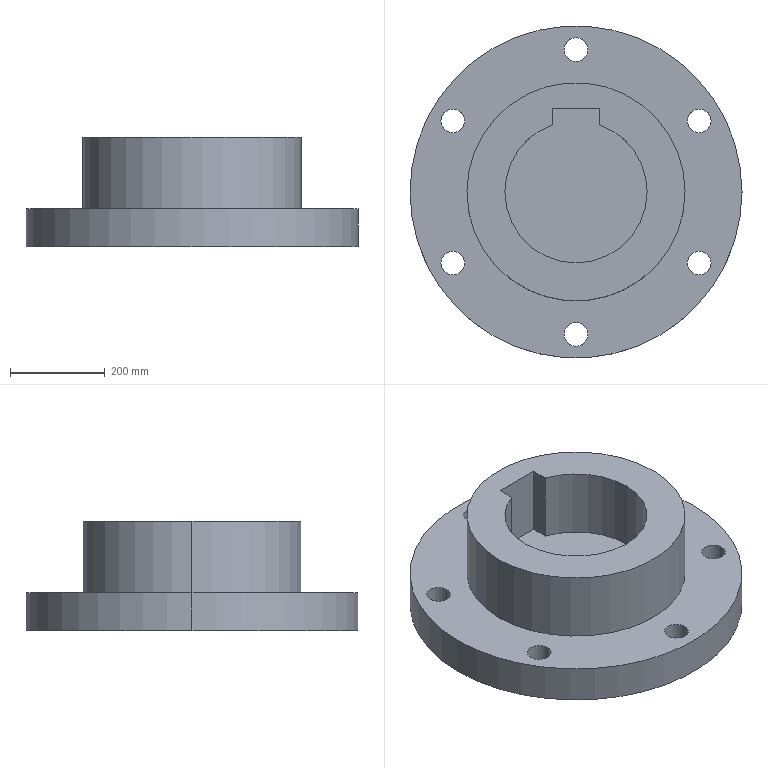Part | SolidWorks | features ICE 2, Extrusion 1 | 1 solid | 26 faces | box 700 x 700 x 230 mm | volume 43732082 mm3 | cylinder 19 | plane 7 | commonest cylinder face diameters 50 x12 300 x3 460 x2 700 x2
STEP:
#1=CARTESIAN_POINT('',(-284.808,150.,-230.));
#2=VERTEX_POINT('',#1);
#3=CARTESIAN_POINT('',(-234.808,150.,-230.));
#4=VERTEX_POINT('',#3);
#5=CARTESIAN_POINT('',(-259.808,150.,-230.));
#6=DIRECTION('',(0.,0.,1.));
#7=DIRECTION('',(-1.,0.,0.));
#8=AXIS2_PLACEMENT_3D('',#5,#6,#7);
#9=CIRCLE('',#8,25.);
#10=EDGE_CURVE('',#2,#4,#9,.T.);
#11=ORIENTED_EDGE('',*,*,#10,.F.);
#12=CARTESIAN_POINT('',(-284.808,150.,-150.));
#13=VERTEX_POINT('',#12);
#14=CARTESIAN_POINT('',(-284.808,150.,-486.));
#15=DIRECTION('',(0.,0.,1.));
#16=VECTOR('',#15,1000.);
#17=LINE('',#14,#16);
#18=EDGE_CURVE('',#2,#13,#17,.T.);
#19=ORIENTED_EDGE('',*,*,#18,.T.);
#20=CARTESIAN_POINT('',(-234.808,150.,-150.));
#21=VERTEX_POINT('',#20);
#22=CARTESIAN_POINT('',(-259.808,150.,-150.));
#23=DIRECTION('',(0.,0.,1.));
#24=DIRECTION('',(-1.,0.,0.));
#25=AXIS2_PLACEMENT_3D('',#22,#23,#24);
#26=CIRCLE('',#25,25.);
#27=EDGE_CURVE('',#13,#21,#26,.T.);
#28=ORIENTED_EDGE('',*,*,#27,.T.);
#29=CARTESIAN_POINT('',(-234.808,150.,-486.));
#30=DIRECTION('',(0.,0.,1.));
#31=VECTOR('',#30,1000.);
#32=LINE('',#29,#31);
#33=EDGE_CURVE('',#4,#21,#32,.T.);
#34=ORIENTED_EDGE('',*,*,#33,.F.);
#35=EDGE_LOOP('',(#11,#19,#28,#34));
#36=FACE_OUTER_BOUND('',#35,.T.);
#37=CARTESIAN_POINT('',(-259.808,150.,-486.));
#38=DIRECTION('',(0.,0.,1.));
#39=DIRECTION('',(1.,0.,0.));
#40=AXIS2_PLACEMENT_3D('',#37,#38,#39);
#41=CYLINDRICAL_SURFACE('',#40,25.);
#42=ADVANCED_FACE('',(#36),#41,.F.);
#43=CARTESIAN_POINT('',(-284.808,-150.,-230.));
#44=VERTEX_POINT('',#43);
#45=CARTESIAN_POINT('',(-234.808,-150.,-230.));
#46=VERTEX_POINT('',#45);
#47=CARTESIAN_POINT('',(-259.808,-150.,-230.));
#48=DIRECTION('',(0.,0.,1.));
#49=DIRECTION('',(-1.,0.,0.));
#50=AXIS2_PLACEMENT_3D('',#47,#48,#49);
#51=CIRCLE('',#50,25.);
#52=EDGE_CURVE('',#44,#46,#51,.T.);
#53=ORIENTED_EDGE('',*,*,#52,.F.);
#54=CARTESIAN_POINT('',(-284.808,-150.,-150.));
#55=VERTEX_POINT('',#54);
#56=CARTESIAN_POINT('',(-284.808,-150.,-486.));
#57=DIRECTION('',(0.,0.,1.));
#58=VECTOR('',#57,1000.);
#59=LINE('',#56,#58);
#60=EDGE_CURVE('',#44,#55,#59,.T.);
#61=ORIENTED_EDGE('',*,*,#60,.T.);
#62=CARTESIAN_POINT('',(-234.808,-150.,-150.));
#63=VERTEX_POINT('',#62);
#64=CARTESIAN_POINT('',(-259.808,-150.,-150.));
#65=DIRECTION('',(0.,0.,1.));
#66=DIRECTION('',(-1.,0.,0.));
#67=AXIS2_PLACEMENT_3D('',#64,#65,#66);
#68=CIRCLE('',#67,25.);
#69=EDGE_CURVE('',#55,#63,#68,.T.);
#70=ORIENTED_EDGE('',*,*,#69,.T.);
#71=CARTESIAN_POINT('',(-234.808,-150.,-486.));
#72=DIRECTION('',(0.,0.,1.));
#73=VECTOR('',#72,1000.);
#74=LINE('',#71,#73);
#75=EDGE_CURVE('',#46,#63,#74,.T.);
#76=ORIENTED_EDGE('',*,*,#75,.F.);
#77=EDGE_LOOP('',(#53,#61,#70,#76));
#78=FACE_OUTER_BOUND('',#77,.T.);
#79=CARTESIAN_POINT('',(-259.808,-150.,-486.));
#80=DIRECTION('',(0.,0.,1.));
#81=DIRECTION('',(1.,0.,0.));
#82=AXIS2_PLACEMENT_3D('',#79,#80,#81);
#83=CYLINDRICAL_SURFACE('',#82,25.);
#84=ADVANCED_FACE('',(#78),#83,.F.);
#85=CARTESIAN_POINT('',(-25.,-300.,-230.));
#86=VERTEX_POINT('',#85);
#87=CARTESIAN_POINT('',(25.,-300.,-230.));
#88=VERTEX_POINT('',#87);
#89=CARTESIAN_POINT('',(0.,-300.,-230.));
#90=DIRECTION('',(0.,0.,1.));
#91=DIRECTION('',(-1.,0.,0.));
#92=AXIS2_PLACEMENT_3D('',#89,#90,#91);
#93=CIRCLE('',#92,25.);
#94=EDGE_CURVE('',#86,#88,#93,.T.);
#95=ORIENTED_EDGE('',*,*,#94,.F.);
#96=CARTESIAN_POINT('',(-25.,-300.,-150.));
#97=VERTEX_POINT('',#96);
#98=CARTESIAN_POINT('',(-25.,-300.,-486.));
#99=DIRECTION('',(0.,0.,1.));
#100=VECTOR('',#99,1000.);
#101=LINE('',#98,#100);
#102=EDGE_CURVE('',#86,#97,#101,.T.);
#103=ORIENTED_EDGE('',*,*,#102,.T.);
#104=CARTESIAN_POINT('',(25.,-300.,-150.));
#105=VERTEX_POINT('',#104);
#106=CARTESIAN_POINT('',(0.,-300.,-150.));
#107=DIRECTION('',(0.,0.,1.));
#108=DIRECTION('',(-1.,0.,0.));
#109=AXIS2_PLACEMENT_3D('',#106,#107,#108);
#110=CIRCLE('',#109,25.);
#111=EDGE_CURVE('',#97,#105,#110,.T.);
#112=ORIENTED_EDGE('',*,*,#111,.T.);
#113=CARTESIAN_POINT('',(25.,-300.,-486.));
#114=DIRECTION('',(0.,0.,1.));
#115=VECTOR('',#114,1000.);
#116=LINE('',#113,#115);
#117=EDGE_CURVE('',#88,#105,#116,.T.);
#118=ORIENTED_EDGE('',*,*,#117,.F.);
#119=EDGE_LOOP('',(#95,#103,#112,#118));
#120=FACE_OUTER_BOUND('',#119,.T.);
#121=CARTESIAN_POINT('',(0.,-300.,-486.));
#122=DIRECTION('',(0.,0.,1.));
#123=DIRECTION('',(1.,0.,0.));
#124=AXIS2_PLACEMENT_3D('',#121,#122,#123);
#125=CYLINDRICAL_SURFACE('',#124,25.);
#126=ADVANCED_FACE('',(#120),#125,.F.);
#127=CARTESIAN_POINT('',(234.808,-150.,-230.));
#128=VERTEX_POINT('',#127);
#129=CARTESIAN_POINT('',(284.808,-150.,-230.));
#130=VERTEX_POINT('',#129);
#131=CARTESIAN_POINT('',(259.808,-150.,-230.));
#132=DIRECTION('',(0.,0.,1.));
#133=DIRECTION('',(-1.,0.,0.));
#134=AXIS2_PLACEMENT_3D('',#131,#132,#133);
#135=CIRCLE('',#134,25.);
#136=EDGE_CURVE('',#128,#130,#135,.T.);
#137=ORIENTED_EDGE('',*,*,#136,.F.);
#138=CARTESIAN_POINT('',(234.808,-150.,-150.));
#139=VERTEX_POINT('',#138);
#140=CARTESIAN_POINT('',(234.808,-150.,-486.));
#141=DIRECTION('',(0.,0.,1.));
#142=VECTOR('',#141,1000.);
#143=LINE('',#140,#142);
#144=EDGE_CURVE('',#128,#139,#143,.T.);
#145=ORIENTED_EDGE('',*,*,#144,.T.);
#146=CARTESIAN_POINT('',(284.808,-150.,-150.));
#147=VERTEX_POINT('',#146);
#148=CARTESIAN_POINT('',(259.808,-150.,-150.));
#149=DIRECTION('',(0.,0.,1.));
#150=DIRECTION('',(-1.,0.,0.));
#151=AXIS2_PLACEMENT_3D('',#148,#149,#150);
#152=CIRCLE('',#151,25.);
#153=EDGE_CURVE('',#139,#147,#152,.T.);
#154=ORIENTED_EDGE('',*,*,#153,.T.);
#155=CARTESIAN_POINT('',(284.808,-150.,-486.));
#156=DIRECTION('',(0.,0.,1.));
#157=VECTOR('',#156,1000.);
#158=LINE('',#155,#157);
#159=EDGE_CURVE('',#130,#147,#158,.T.);
#160=ORIENTED_EDGE('',*,*,#159,.F.);
#161=EDGE_LOOP('',(#137,#145,#154,#160));
#162=FACE_OUTER_BOUND('',#161,.T.);
#163=CARTESIAN_POINT('',(259.808,-150.,-486.));
#164=DIRECTION('',(0.,0.,1.));
#165=DIRECTION('',(1.,0.,0.));
#166=AXIS2_PLACEMENT_3D('',#163,#164,#165);
#167=CYLINDRICAL_SURFACE('',#166,25.);
#168=ADVANCED_FACE('',(#162),#167,.F.);
#169=CARTESIAN_POINT('',(234.808,150.,-230.));
#170=VERTEX_POINT('',#169);
#171=CARTESIAN_POINT('',(284.808,150.,-230.));
#172=VERTEX_POINT('',#171);
#173=CARTESIAN_POINT('',(259.808,150.,-230.));
#174=DIRECTION('',(0.,0.,1.));
#175=DIRECTION('',(-1.,0.,0.));
#176=AXIS2_PLACEMENT_3D('',#173,#174,#175);
#177=CIRCLE('',#176,25.);
#178=EDGE_CURVE('',#170,#172,#177,.T.);
#179=ORIENTED_EDGE('',*,*,#178,.F.);
#180=CARTESIAN_POINT('',(234.808,150.,-150.));
#181=VERTEX_POINT('',#180);
#182=CARTESIAN_POINT('',(234.808,150.,-486.));
#183=DIRECTION('',(0.,0.,1.));
#184=VECTOR('',#183,1000.);
#185=LINE('',#182,#184);
#186=EDGE_CURVE('',#170,#181,#185,.T.);
#187=ORIENTED_EDGE('',*,*,#186,.T.);
#188=CARTESIAN_POINT('',(284.808,150.,-150.));
#189=VERTEX_POINT('',#188);
#190=CARTESIAN_POINT('',(259.808,150.,-150.));
#191=DIRECTION('',(0.,0.,1.));
#192=DIRECTION('',(-1.,0.,0.));
#193=AXIS2_PLACEMENT_3D('',#190,#191,#192);
#194=CIRCLE('',#193,25.);
#195=EDGE_CURVE('',#181,#189,#194,.T.);
#196=ORIENTED_EDGE('',*,*,#195,.T.);
#197=CARTESIAN_POINT('',(284.808,150.,-486.));
#198=DIRECTION('',(0.,0.,1.));
#199=VECTOR('',#198,1000.);
#200=LINE('',#197,#199);
#201=EDGE_CURVE('',#172,#189,#200,.T.);
#202=ORIENTED_EDGE('',*,*,#201,.F.);
#203=EDGE_LOOP('',(#179,#187,#196,#202));
#204=FACE_OUTER_BOUND('',#203,.T.);
#205=CARTESIAN_POINT('',(259.808,150.,-486.));
#206=DIRECTION('',(0.,0.,1.));
#207=DIRECTION('',(1.,0.,0.));
#208=AXIS2_PLACEMENT_3D('',#205,#206,#207);
#209=CYLINDRICAL_SURFACE('',#208,25.);
#210=ADVANCED_FACE('',(#204),#209,.F.);
#211=CARTESIAN_POINT('',(-25.,300.,-230.));
#212=VERTEX_POINT('',#211);
#213=CARTESIAN_POINT('',(25.,300.,-230.));
#214=VERTEX_POINT('',#213);
#215=CARTESIAN_POINT('',(0.,300.,-230.));
#216=DIRECTION('',(0.,0.,1.));
#217=DIRECTION('',(-1.,0.,0.));
#218=AXIS2_PLACEMENT_3D('',#215,#216,#217);
#219=CIRCLE('',#218,25.);
#220=EDGE_CURVE('',#212,#214,#219,.T.);
#221=ORIENTED_EDGE('',*,*,#220,.F.);
#222=CARTESIAN_POINT('',(-25.,300.,-150.));
#223=VERTEX_POINT('',#222);
#224=CARTESIAN_POINT('',(-25.,300.,-486.));
#225=DIRECTION('',(0.,0.,1.));
#226=VECTOR('',#225,1000.);
#227=LINE('',#224,#226);
#228=EDGE_CURVE('',#212,#223,#227,.T.);
#229=ORIENTED_EDGE('',*,*,#228,.T.);
#230=CARTESIAN_POINT('',(25.,300.,-150.));
#231=VERTEX_POINT('',#230);
#232=CARTESIAN_POINT('',(0.,300.,-150.));
#233=DIRECTION('',(0.,0.,1.));
#234=DIRECTION('',(-1.,0.,0.));
#235=AXIS2_PLACEMENT_3D('',#232,#233,#234);
#236=CIRCLE('',#235,25.);
#237=EDGE_CURVE('',#223,#231,#236,.T.);
#238=ORIENTED_EDGE('',*,*,#237,.T.);
#239=CARTESIAN_POINT('',(25.,300.,-486.));
#240=DIRECTION('',(0.,0.,1.));
#241=VECTOR('',#240,1000.);
#242=LINE('',#239,#241);
#243=EDGE_CURVE('',#214,#231,#242,.T.);
#244=ORIENTED_EDGE('',*,*,#243,.F.);
#245=EDGE_LOOP('',(#221,#229,#238,#244));
#246=FACE_OUTER_BOUND('',#245,.T.);
#247=CARTESIAN_POINT('',(0.,300.,-486.));
#248=DIRECTION('',(0.,0.,1.));
#249=DIRECTION('',(1.,0.,0.));
#250=AXIS2_PLACEMENT_3D('',#247,#248,#249);
#251=CYLINDRICAL_SURFACE('',#250,25.);
#252=ADVANCED_FACE('',(#246),#251,.F.);
#253=CARTESIAN_POINT('',(-350.,0.,-230.));
#254=VERTEX_POINT('',#253);
#255=CARTESIAN_POINT('',(350.,0.,-230.));
#256=VERTEX_POINT('',#255);
#257=CARTESIAN_POINT('',(0.,0.,-230.));
#258=DIRECTION('',(0.,0.,-1.));
#259=DIRECTION('',(-1.,0.,0.));
#260=AXIS2_PLACEMENT_3D('',#257,#258,#259);
#261=CIRCLE('',#260,350.);
#262=EDGE_CURVE('',#254,#256,#261,.T.);
#263=ORIENTED_EDGE('',*,*,#262,.F.);
#264=CARTESIAN_POINT('',(-350.,0.,-150.));
#265=VERTEX_POINT('',#264);
#266=CARTESIAN_POINT('',(-350.,0.,-230.));
#267=DIRECTION('',(0.,0.,1.));
#268=VECTOR('',#267,1000.);
#269=LINE('',#266,#268);
#270=EDGE_CURVE('',#254,#265,#269,.T.);
#271=ORIENTED_EDGE('',*,*,#270,.T.);
#272=CARTESIAN_POINT('',(350.,0.,-150.));
#273=VERTEX_POINT('',#272);
#274=CARTESIAN_POINT('',(0.,0.,-150.));
#275=DIRECTION('',(0.,0.,-1.));
#276=DIRECTION('',(-1.,0.,0.));
#277=AXIS2_PLACEMENT_3D('',#274,#275,#276);
#278=CIRCLE('',#277,350.);
#279=EDGE_CURVE('',#265,#273,#278,.T.);
#280=ORIENTED_EDGE('',*,*,#279,.T.);
#281=CARTESIAN_POINT('',(350.,0.,-230.));
#282=DIRECTION('',(0.,0.,1.));
#283=VECTOR('',#282,1000.);
#284=LINE('',#281,#283);
#285=EDGE_CURVE('',#256,#273,#284,.T.);
#286=ORIENTED_EDGE('',*,*,#285,.F.);
#287=EDGE_LOOP('',(#263,#271,#280,#286));
#288=FACE_OUTER_BOUND('',#287,.T.);
#289=CARTESIAN_POINT('',(0.,0.,-230.));
#290=DIRECTION('',(0.,0.,1.));
#291=DIRECTION('',(1.,0.,0.));
#292=AXIS2_PLACEMENT_3D('',#289,#290,#291);
#293=CYLINDRICAL_SURFACE('',#292,350.);
#294=ADVANCED_FACE('',(#288),#293,.T.);
#295=CARTESIAN_POINT('',(-150.,0.,-150.));
#296=VERTEX_POINT('',#295);
#297=CARTESIAN_POINT('',(150.,0.,-150.));
#298=VERTEX_POINT('',#297);
#299=CARTESIAN_POINT('',(0.,0.,-150.));
#300=DIRECTION('',(0.,0.,1.));
#301=DIRECTION('',(1.,0.,0.));
#302=AXIS2_PLACEMENT_3D('',#299,#300,#301);
#303=CIRCLE('',#302,150.);
#304=EDGE_CURVE('',#296,#298,#303,.T.);
#305=ORIENTED_EDGE('',*,*,#304,.F.);
#306=CARTESIAN_POINT('',(-150.,0.,0.));
#307=VERTEX_POINT('',#306);
#308=CARTESIAN_POINT('',(-150.,0.,-150.));
#309=DIRECTION('',(0.,0.,1.));
#310=VECTOR('',#309,1000.);
#311=LINE('',#308,#310);
#312=EDGE_CURVE('',#296,#307,#311,.T.);
#313=ORIENTED_EDGE('',*,*,#312,.T.);
#314=CARTESIAN_POINT('',(150.,0.,0.));
#315=VERTEX_POINT('',#314);
#316=CARTESIAN_POINT('',(0.,0.,0.));
#317=DIRECTION('',(0.,0.,1.));
#318=DIRECTION('',(1.,0.,0.));
#319=AXIS2_PLACEMENT_3D('',#316,#317,#318);
#320=CIRCLE('',#319,150.);
#321=EDGE_CURVE('',#307,#315,#320,.T.);
#322=ORIENTED_EDGE('',*,*,#321,.T.);
#323=CARTESIAN_POINT('',(150.,0.,-150.));
#324=DIRECTION('',(0.,0.,1.));
#325=VECTOR('',#324,1000.);
#326=LINE('',#323,#325);
#327=EDGE_CURVE('',#298,#315,#326,.T.);
#328=ORIENTED_EDGE('',*,*,#327,.F.);
#329=EDGE_LOOP('',(#305,#313,#322,#328));
#330=FACE_OUTER_BOUND('',#329,.T.);
#331=CARTESIAN_POINT('',(0.,0.,-150.));
#332=DIRECTION('',(0.,0.,1.));
#333=DIRECTION('',(1.,0.,0.));
#334=AXIS2_PLACEMENT_3D('',#331,#332,#333);
#335=CYLINDRICAL_SURFACE('',#334,150.);
#336=ADVANCED_FACE('',(#330),#335,.F.);
#337=CARTESIAN_POINT('',(50.,141.421,-150.));
#338=VERTEX_POINT('',#337);
#339=CARTESIAN_POINT('',(0.,0.,-150.));
#340=DIRECTION('',(0.,0.,1.));
#341=DIRECTION('',(1.,0.,0.));
#342=AXIS2_PLACEMENT_3D('',#339,#340,#341);
#343=CIRCLE('',#342,150.);
#344=EDGE_CURVE('',#298,#338,#343,.T.);
#345=ORIENTED_EDGE('',*,*,#344,.F.);
#346=ORIENTED_EDGE('',*,*,#327,.T.);
#347=CARTESIAN_POINT('',(50.,141.421,0.));
#348=VERTEX_POINT('',#347);
#349=CARTESIAN_POINT('',(0.,0.,0.));
#350=DIRECTION('',(0.,0.,1.));
#351=DIRECTION('',(1.,0.,0.));
#352=AXIS2_PLACEMENT_3D('',#349,#350,#351);
#353=CIRCLE('',#352,150.);
#354=EDGE_CURVE('',#315,#348,#353,.T.);
#355=ORIENTED_EDGE('',*,*,#354,.T.);
#356=CARTESIAN_POINT('',(50.,141.421,-150.));
#357=DIRECTION('',(0.,0.,1.));
#358=VECTOR('',#357,1000.);
#359=LINE('',#356,#358);
#360=EDGE_CURVE('',#338,#348,#359,.T.);
#361=ORIENTED_EDGE('',*,*,#360,.F.);
#362=EDGE_LOOP('',(#345,#346,#355,#361));
#363=FACE_OUTER_BOUND('',#362,.T.);
#364=CARTESIAN_POINT('',(0.,0.,-150.));
#365=DIRECTION('',(0.,0.,1.));
#366=DIRECTION('',(1.,0.,0.));
#367=AXIS2_PLACEMENT_3D('',#364,#365,#366);
#368=CYLINDRICAL_SURFACE('',#367,150.);
#369=ADVANCED_FACE('',(#363),#368,.F.);
#370=CARTESIAN_POINT('',(230.,0.,-150.));
#371=VERTEX_POINT('',#370);
#372=CARTESIAN_POINT('',(-230.,0.,-150.));
#373=VERTEX_POINT('',#372);
#374=CARTESIAN_POINT('',(0.,0.,-150.));
#375=DIRECTION('',(0.,0.,1.));
#376=DIRECTION('',(-1.,0.,0.));
#377=AXIS2_PLACEMENT_3D('',#374,#375,#376);
#378=CIRCLE('',#377,230.);
#379=EDGE_CURVE('',#371,#373,#378,.T.);
#380=ORIENTED_EDGE('',*,*,#379,.T.);
#381=CARTESIAN_POINT('',(-230.,0.,0.));
#382=VERTEX_POINT('',#381);
#383=CARTESIAN_POINT('',(-230.,0.,-150.));
#384=DIRECTION('',(0.,0.,1.));
#385=VECTOR('',#384,1000.);
#386=LINE('',#383,#385);
#387=EDGE_CURVE('',#373,#382,#386,.T.);
#388=ORIENTED_EDGE('',*,*,#387,.T.);
#389=CARTESIAN_POINT('',(230.,0.,0.));
#390=VERTEX_POINT('',#389);
#391=CARTESIAN_POINT('',(0.,0.,0.));
#392=DIRECTION('',(0.,0.,1.));
#393=DIRECTION('',(1.,0.,0.));
#394=AXIS2_PLACEMENT_3D('',#391,#392,#393);
#395=CIRCLE('',#394,230.);
#396=EDGE_CURVE('',#390,#382,#395,.T.);
#397=ORIENTED_EDGE('',*,*,#396,.F.);
#398=CARTESIAN_POINT('',(230.,0.,-150.));
#399=DIRECTION('',(0.,0.,1.));
#400=VECTOR('',#399,1000.);
#401=LINE('',#398,#400);
#402=EDGE_CURVE('',#371,#390,#401,.T.);
#403=ORIENTED_EDGE('',*,*,#402,.F.);
#404=EDGE_LOOP('',(#380,#388,#397,#403));
#405=FACE_OUTER_BOUND('',#404,.T.);
#406=CARTESIAN_POINT('',(0.,0.,-150.));
#407=DIRECTION('',(0.,0.,1.));
#408=DIRECTION('',(1.,0.,0.));
#409=AXIS2_PLACEMENT_3D('',#406,#407,#408);
#410=CYLINDRICAL_SURFACE('',#409,230.);
#411=ADVANCED_FACE('',(#405),#410,.T.);
#412=ORIENTED_EDGE('',*,*,#387,.F.);
#413=CARTESIAN_POINT('',(0.,0.,-150.));
#414=DIRECTION('',(0.,0.,1.));
#415=DIRECTION('',(-1.,0.,0.));
#416=AXIS2_PLACEMENT_3D('',#413,#414,#415);
#417=CIRCLE('',#416,230.);
#418=EDGE_CURVE('',#373,#371,#417,.T.);
#419=ORIENTED_EDGE('',*,*,#418,.T.);
#420=ORIENTED_EDGE('',*,*,#402,.T.);
#421=CARTESIAN_POINT('',(0.,0.,0.));
#422=DIRECTION('',(0.,0.,1.));
#423=DIRECTION('',(1.,0.,0.));
#424=AXIS2_PLACEMENT_3D('',#421,#422,#423);
#425=CIRCLE('',#424,230.);
#426=EDGE_CURVE('',#382,#390,#425,.T.);
#427=ORIENTED_EDGE('',*,*,#426,.F.);
#428=EDGE_LOOP('',(#412,#419,#420,#427));
#429=FACE_OUTER_BOUND('',#428,.T.);
#430=CARTESIAN_POINT('',(0.,0.,-150.));
#431=DIRECTION('',(0.,0.,1.));
#432=DIRECTION('',(1.,0.,0.));
#433=AXIS2_PLACEMENT_3D('',#430,#431,#432);
#434=CYLINDRICAL_SURFACE('',#433,230.);
#435=ADVANCED_FACE('',(#429),#434,.T.);
#436=CARTESIAN_POINT('',(-50.,141.421,0.));
#437=VERTEX_POINT('',#436);
#438=CARTESIAN_POINT('',(0.,0.,0.));
#439=DIRECTION('',(0.,0.,1.));
#440=DIRECTION('',(1.,0.,0.));
#441=AXIS2_PLACEMENT_3D('',#438,#439,#440);
#442=CIRCLE('',#441,150.);
#443=EDGE_CURVE('',#437,#307,#442,.T.);
#444=ORIENTED_EDGE('',*,*,#443,.F.);
#445=CARTESIAN_POINT('',(-50.,176.421,0.));
#446=VERTEX_POINT('',#445);
#447=CARTESIAN_POINT('',(-50.,141.421,0.));
#448=DIRECTION('',(0.,-1.,0.));
#449=VECTOR('',#448,1000.);
#450=LINE('',#447,#449);
#451=EDGE_CURVE('',#446,#437,#450,.T.);
#452=ORIENTED_EDGE('',*,*,#451,.F.);
#453=CARTESIAN_POINT('',(50.,176.421,0.));
#454=VERTEX_POINT('',#453);
#455=CARTESIAN_POINT('',(-50.,176.421,0.));
#456=DIRECTION('',(-1.,0.,0.));
#457=VECTOR('',#456,1000.);
#458=LINE('',#455,#457);
#459=EDGE_CURVE('',#454,#446,#458,.T.);
#460=ORIENTED_EDGE('',*,*,#459,.F.);
#461=CARTESIAN_POINT('',(50.,141.421,0.));
#462=DIRECTION('',(0.,1.,0.));
#463=VECTOR('',#462,1000.);
#464=LINE('',#461,#463);
#465=EDGE_CURVE('',#348,#454,#464,.T.);
#466=ORIENTED_EDGE('',*,*,#465,.F.);
#467=ORIENTED_EDGE('',*,*,#354,.F.);
#468=ORIENTED_EDGE('',*,*,#321,.F.);
#469=EDGE_LOOP('',(#444,#452,#460,#466,#467,#468));
#470=FACE_BOUND('',#469,.T.);
#471=ORIENTED_EDGE('',*,*,#396,.T.);
#472=ORIENTED_EDGE('',*,*,#426,.T.);
#473=EDGE_LOOP('',(#471,#472));
#474=FACE_OUTER_BOUND('',#473,.T.);
#475=CARTESIAN_POINT('',(0.,0.,0.));
#476=DIRECTION('',(0.,0.,1.));
#477=DIRECTION('',(1.,0.,0.));
#478=AXIS2_PLACEMENT_3D('',#475,#476,#477);
#479=PLANE('',#478);
#480=ADVANCED_FACE('',(#470,#474),#479,.T.);
#481=ORIENTED_EDGE('',*,*,#312,.F.);
#482=CARTESIAN_POINT('',(-50.,141.421,-150.));
#483=VERTEX_POINT('',#482);
#484=CARTESIAN_POINT('',(0.,0.,-150.));
#485=DIRECTION('',(0.,0.,1.));
#486=DIRECTION('',(1.,0.,0.));
#487=AXIS2_PLACEMENT_3D('',#484,#485,#486);
#488=CIRCLE('',#487,150.);
#489=EDGE_CURVE('',#483,#296,#488,.T.);
#490=ORIENTED_EDGE('',*,*,#489,.F.);
#491=CARTESIAN_POINT('',(-50.,141.421,-150.));
#492=DIRECTION('',(0.,0.,1.));
#493=VECTOR('',#492,1000.);
#494=LINE('',#491,#493);
#495=EDGE_CURVE('',#483,#437,#494,.T.);
#496=ORIENTED_EDGE('',*,*,#495,.T.);
#497=ORIENTED_EDGE('',*,*,#443,.T.);
#498=EDGE_LOOP('',(#481,#490,#496,#497));
#499=FACE_OUTER_BOUND('',#498,.T.);
#500=CARTESIAN_POINT('',(0.,0.,-150.));
#501=DIRECTION('',(0.,0.,1.));
#502=DIRECTION('',(1.,0.,0.));
#503=AXIS2_PLACEMENT_3D('',#500,#501,#502);
#504=CYLINDRICAL_SURFACE('',#503,150.);
#505=ADVANCED_FACE('',(#499),#504,.F.);
#506=ORIENTED_EDGE('',*,*,#451,.T.);
#507=ORIENTED_EDGE('',*,*,#495,.F.);
#508=CARTESIAN_POINT('',(-50.,176.421,-150.));
#509=VERTEX_POINT('',#508);
#510=CARTESIAN_POINT('',(-50.,141.421,-150.));
#511=DIRECTION('',(0.,-1.,0.));
#512=VECTOR('',#511,1000.);
#513=LINE('',#510,#512);
#514=EDGE_CURVE('',#509,#483,#513,.T.);
#515=ORIENTED_EDGE('',*,*,#514,.F.);
#516=CARTESIAN_POINT('',(-50.,176.421,-150.));
#517=DIRECTION('',(0.,0.,1.));
#518=VECTOR('',#517,1000.);
#519=LINE('',#516,#518);
#520=EDGE_CURVE('',#509,#446,#519,.T.);
#521=ORIENTED_EDGE('',*,*,#520,.T.);
#522=EDGE_LOOP('',(#506,#507,#515,#521));
#523=FACE_OUTER_BOUND('',#522,.T.);
#524=CARTESIAN_POINT('',(-50.,141.421,-150.));
#525=DIRECTION('',(-1.,0.,0.));
#526=DIRECTION('',(0.,-1.,0.));
#527=AXIS2_PLACEMENT_3D('',#524,#525,#526);
#528=PLANE('',#527);
#529=ADVANCED_FACE('',(#523),#528,.F.);
#530=ORIENTED_EDGE('',*,*,#459,.T.);
#531=ORIENTED_EDGE('',*,*,#520,.F.);
#532=CARTESIAN_POINT('',(50.,176.421,-150.));
#533=VERTEX_POINT('',#532);
#534=CARTESIAN_POINT('',(-50.,176.421,-150.));
#535=DIRECTION('',(-1.,0.,0.));
#536=VECTOR('',#535,1000.);
#537=LINE('',#534,#536);
#538=EDGE_CURVE('',#533,#509,#537,.T.);
#539=ORIENTED_EDGE('',*,*,#538,.F.);
#540=CARTESIAN_POINT('',(50.,176.421,-150.));
#541=DIRECTION('',(0.,0.,1.));
#542=VECTOR('',#541,1000.);
#543=LINE('',#540,#542);
#544=EDGE_CURVE('',#533,#454,#543,.T.);
#545=ORIENTED_EDGE('',*,*,#544,.T.);
#546=EDGE_LOOP('',(#530,#531,#539,#545));
#547=FACE_OUTER_BOUND('',#546,.T.);
#548=CARTESIAN_POINT('',(-50.,176.421,-150.));
#549=DIRECTION('',(0.,1.,0.));
#550=DIRECTION('',(0.,0.,1.));
#551=AXIS2_PLACEMENT_3D('',#548,#549,#550);
#552=PLANE('',#551);
#553=ADVANCED_FACE('',(#547),#552,.F.);
#554=ORIENTED_EDGE('',*,*,#465,.T.);
#555=ORIENTED_EDGE('',*,*,#544,.F.);
#556=CARTESIAN_POINT('',(50.,141.421,-150.));
#557=DIRECTION('',(0.,1.,0.));
#558=VECTOR('',#557,1000.);
#559=LINE('',#556,#558);
#560=EDGE_CURVE('',#338,#533,#559,.T.);
#561=ORIENTED_EDGE('',*,*,#560,.F.);
#562=ORIENTED_EDGE('',*,*,#360,.T.);
#563=EDGE_LOOP('',(#554,#555,#561,#562));
#564=FACE_OUTER_BOUND('',#563,.T.);
#565=CARTESIAN_POINT('',(50.,141.421,-150.));
#566=DIRECTION('',(1.,0.,0.));
#567=DIRECTION('',(0.,1.,0.));
#568=AXIS2_PLACEMENT_3D('',#565,#566,#567);
#569=PLANE('',#568);
#570=ADVANCED_FACE('',(#564),#569,.F.);
#571=ORIENTED_EDGE('',*,*,#514,.T.);
#572=ORIENTED_EDGE('',*,*,#489,.T.);
#573=ORIENTED_EDGE('',*,*,#304,.T.);
#574=ORIENTED_EDGE('',*,*,#344,.T.);
#575=ORIENTED_EDGE('',*,*,#560,.T.);
#576=ORIENTED_EDGE('',*,*,#538,.T.);
#577=EDGE_LOOP('',(#571,#572,#573,#574,#575,#576));
#578=FACE_OUTER_BOUND('',#577,.T.);
#579=CARTESIAN_POINT('',(0.,0.,-150.));
#580=DIRECTION('',(0.,0.,-1.));
#581=DIRECTION('',(-1.,0.,0.));
#582=AXIS2_PLACEMENT_3D('',#579,#580,#581);
#583=PLANE('',#582);
#584=ADVANCED_FACE('',(#578),#583,.F.);
#585=ORIENTED_EDGE('',*,*,#270,.F.);
#586=CARTESIAN_POINT('',(0.,0.,-230.));
#587=DIRECTION('',(0.,0.,-1.));
#588=DIRECTION('',(-1.,0.,0.));
#589=AXIS2_PLACEMENT_3D('',#586,#587,#588);
#590=CIRCLE('',#589,350.);
#591=EDGE_CURVE('',#256,#254,#590,.T.);
#592=ORIENTED_EDGE('',*,*,#591,.F.);
#593=ORIENTED_EDGE('',*,*,#285,.T.);
#594=CARTESIAN_POINT('',(0.,0.,-150.));
#595=DIRECTION('',(0.,0.,-1.));
#596=DIRECTION('',(-1.,0.,0.));
#597=AXIS2_PLACEMENT_3D('',#594,#595,#596);
#598=CIRCLE('',#597,350.);
#599=EDGE_CURVE('',#273,#265,#598,.T.);
#600=ORIENTED_EDGE('',*,*,#599,.T.);
#601=EDGE_LOOP('',(#585,#592,#593,#600));
#602=FACE_OUTER_BOUND('',#601,.T.);
#603=CARTESIAN_POINT('',(0.,0.,-230.));
#604=DIRECTION('',(0.,0.,1.));
#605=DIRECTION('',(1.,0.,0.));
#606=AXIS2_PLACEMENT_3D('',#603,#604,#605);
#607=CYLINDRICAL_SURFACE('',#606,350.);
#608=ADVANCED_FACE('',(#602),#607,.T.);
#609=CARTESIAN_POINT('',(-259.808,150.,-230.));
#610=DIRECTION('',(0.,0.,1.));
#611=DIRECTION('',(-1.,0.,0.));
#612=AXIS2_PLACEMENT_3D('',#609,#610,#611);
#613=CIRCLE('',#612,25.);
#614=EDGE_CURVE('',#4,#2,#613,.T.);
#615=ORIENTED_EDGE('',*,*,#614,.T.);
#616=ORIENTED_EDGE('',*,*,#10,.T.);
#617=EDGE_LOOP('',(#615,#616));
#618=FACE_BOUND('',#617,.T.);
#619=CARTESIAN_POINT('',(-259.808,-150.,-230.));
#620=DIRECTION('',(0.,0.,1.));
#621=DIRECTION('',(-1.,0.,0.));
#622=AXIS2_PLACEMENT_3D('',#619,#620,#621);
#623=CIRCLE('',#622,25.);
#624=EDGE_CURVE('',#46,#44,#623,.T.);
#625=ORIENTED_EDGE('',*,*,#624,.T.);
#626=ORIENTED_EDGE('',*,*,#52,.T.);
#627=EDGE_LOOP('',(#625,#626));
#628=FACE_BOUND('',#627,.T.);
#629=CARTESIAN_POINT('',(0.,-300.,-230.));
#630=DIRECTION('',(0.,0.,1.));
#631=DIRECTION('',(-1.,0.,0.));
#632=AXIS2_PLACEMENT_3D('',#629,#630,#631);
#633=CIRCLE('',#632,25.);
#634=EDGE_CURVE('',#88,#86,#633,.T.);
#635=ORIENTED_EDGE('',*,*,#634,.T.);
#636=ORIENTED_EDGE('',*,*,#94,.T.);
#637=EDGE_LOOP('',(#635,#636));
#638=FACE_BOUND('',#637,.T.);
#639=CARTESIAN_POINT('',(259.808,-150.,-230.));
#640=DIRECTION('',(0.,0.,1.));
#641=DIRECTION('',(-1.,0.,0.));
#642=AXIS2_PLACEMENT_3D('',#639,#640,#641);
#643=CIRCLE('',#642,25.);
#644=EDGE_CURVE('',#130,#128,#643,.T.);
#645=ORIENTED_EDGE('',*,*,#644,.T.);
#646=ORIENTED_EDGE('',*,*,#136,.T.);
#647=EDGE_LOOP('',(#645,#646));
#648=FACE_BOUND('',#647,.T.);
#649=CARTESIAN_POINT('',(259.808,150.,-230.));
#650=DIRECTION('',(0.,0.,1.));
#651=DIRECTION('',(-1.,0.,0.));
#652=AXIS2_PLACEMENT_3D('',#649,#650,#651);
#653=CIRCLE('',#652,25.);
#654=EDGE_CURVE('',#172,#170,#653,.T.);
#655=ORIENTED_EDGE('',*,*,#654,.T.);
#656=ORIENTED_EDGE('',*,*,#178,.T.);
#657=EDGE_LOOP('',(#655,#656));
#658=FACE_BOUND('',#657,.T.);
#659=CARTESIAN_POINT('',(0.,300.,-230.));
#660=DIRECTION('',(0.,0.,1.));
#661=DIRECTION('',(-1.,0.,0.));
#662=AXIS2_PLACEMENT_3D('',#659,#660,#661);
#663=CIRCLE('',#662,25.);
#664=EDGE_CURVE('',#214,#212,#663,.T.);
#665=ORIENTED_EDGE('',*,*,#664,.T.);
#666=ORIENTED_EDGE('',*,*,#220,.T.);
#667=EDGE_LOOP('',(#665,#666));
#668=FACE_BOUND('',#667,.T.);
#669=ORIENTED_EDGE('',*,*,#591,.T.);
#670=ORIENTED_EDGE('',*,*,#262,.T.);
#671=EDGE_LOOP('',(#669,#670));
#672=FACE_OUTER_BOUND('',#671,.T.);
#673=CARTESIAN_POINT('',(0.,0.,-230.));
#674=DIRECTION('',(0.,0.,-1.));
#675=DIRECTION('',(-1.,0.,0.));
#676=AXIS2_PLACEMENT_3D('',#673,#674,#675);
#677=PLANE('',#676);
#678=ADVANCED_FACE('',(#618,#628,#638,#648,#658,#668,#672),#677,.T.);
#679=CARTESIAN_POINT('',(-259.808,150.,-150.));
#680=DIRECTION('',(0.,0.,1.));
#681=DIRECTION('',(-1.,0.,0.));
#682=AXIS2_PLACEMENT_3D('',#679,#680,#681);
#683=CIRCLE('',#682,25.);
#684=EDGE_CURVE('',#21,#13,#683,.T.);
#685=ORIENTED_EDGE('',*,*,#684,.F.);
#686=ORIENTED_EDGE('',*,*,#27,.F.);
#687=EDGE_LOOP('',(#685,#686));
#688=FACE_BOUND('',#687,.T.);
#689=CARTESIAN_POINT('',(-259.808,-150.,-150.));
#690=DIRECTION('',(0.,0.,1.));
#691=DIRECTION('',(-1.,0.,0.));
#692=AXIS2_PLACEMENT_3D('',#689,#690,#691);
#693=CIRCLE('',#692,25.);
#694=EDGE_CURVE('',#63,#55,#693,.T.);
#695=ORIENTED_EDGE('',*,*,#694,.F.);
#696=ORIENTED_EDGE('',*,*,#69,.F.);
#697=EDGE_LOOP('',(#695,#696));
#698=FACE_BOUND('',#697,.T.);
#699=CARTESIAN_POINT('',(0.,-300.,-150.));
#700=DIRECTION('',(0.,0.,1.));
#701=DIRECTION('',(-1.,0.,0.));
#702=AXIS2_PLACEMENT_3D('',#699,#700,#701);
#703=CIRCLE('',#702,25.);
#704=EDGE_CURVE('',#105,#97,#703,.T.);
#705=ORIENTED_EDGE('',*,*,#704,.F.);
#706=ORIENTED_EDGE('',*,*,#111,.F.);
#707=EDGE_LOOP('',(#705,#706));
#708=FACE_BOUND('',#707,.T.);
#709=CARTESIAN_POINT('',(259.808,-150.,-150.));
#710=DIRECTION('',(0.,0.,1.));
#711=DIRECTION('',(-1.,0.,0.));
#712=AXIS2_PLACEMENT_3D('',#709,#710,#711);
#713=CIRCLE('',#712,25.);
#714=EDGE_CURVE('',#147,#139,#713,.T.);
#715=ORIENTED_EDGE('',*,*,#714,.F.);
#716=ORIENTED_EDGE('',*,*,#153,.F.);
#717=EDGE_LOOP('',(#715,#716));
#718=FACE_BOUND('',#717,.T.);
#719=CARTESIAN_POINT('',(259.808,150.,-150.));
#720=DIRECTION('',(0.,0.,1.));
#721=DIRECTION('',(-1.,0.,0.));
#722=AXIS2_PLACEMENT_3D('',#719,#720,#721);
#723=CIRCLE('',#722,25.);
#724=EDGE_CURVE('',#189,#181,#723,.T.);
#725=ORIENTED_EDGE('',*,*,#724,.F.);
#726=ORIENTED_EDGE('',*,*,#195,.F.);
#727=EDGE_LOOP('',(#725,#726));
#728=FACE_BOUND('',#727,.T.);
#729=CARTESIAN_POINT('',(0.,300.,-150.));
#730=DIRECTION('',(0.,0.,1.));
#731=DIRECTION('',(-1.,0.,0.));
#732=AXIS2_PLACEMENT_3D('',#729,#730,#731);
#733=CIRCLE('',#732,25.);
#734=EDGE_CURVE('',#231,#223,#733,.T.);
#735=ORIENTED_EDGE('',*,*,#734,.F.);
#736=ORIENTED_EDGE('',*,*,#237,.F.);
#737=EDGE_LOOP('',(#735,#736));
#738=FACE_BOUND('',#737,.T.);
#739=ORIENTED_EDGE('',*,*,#379,.F.);
#740=ORIENTED_EDGE('',*,*,#418,.F.);
#741=EDGE_LOOP('',(#739,#740));
#742=FACE_BOUND('',#741,.T.);
#743=ORIENTED_EDGE('',*,*,#599,.F.);
#744=ORIENTED_EDGE('',*,*,#279,.F.);
#745=EDGE_LOOP('',(#743,#744));
#746=FACE_OUTER_BOUND('',#745,.T.);
#747=CARTESIAN_POINT('',(0.,0.,-150.));
#748=DIRECTION('',(0.,0.,-1.));
#749=DIRECTION('',(-1.,0.,0.));
#750=AXIS2_PLACEMENT_3D('',#747,#748,#749);
#751=PLANE('',#750);
#752=ADVANCED_FACE('',(#688,#698,#708,#718,#728,#738,#742,#746),#751,.F.);
#753=ORIENTED_EDGE('',*,*,#228,.F.);
#754=ORIENTED_EDGE('',*,*,#664,.F.);
#755=ORIENTED_EDGE('',*,*,#243,.T.);
#756=ORIENTED_EDGE('',*,*,#734,.T.);
#757=EDGE_LOOP('',(#753,#754,#755,#756));
#758=FACE_OUTER_BOUND('',#757,.T.);
#759=CARTESIAN_POINT('',(0.,300.,-486.));
#760=DIRECTION('',(0.,0.,1.));
#761=DIRECTION('',(1.,0.,0.));
#762=AXIS2_PLACEMENT_3D('',#759,#760,#761);
#763=CYLINDRICAL_SURFACE('',#762,25.);
#764=ADVANCED_FACE('',(#758),#763,.F.);
#765=ORIENTED_EDGE('',*,*,#186,.F.);
#766=ORIENTED_EDGE('',*,*,#654,.F.);
#767=ORIENTED_EDGE('',*,*,#201,.T.);
#768=ORIENTED_EDGE('',*,*,#724,.T.);
#769=EDGE_LOOP('',(#765,#766,#767,#768));
#770=FACE_OUTER_BOUND('',#769,.T.);
#771=CARTESIAN_POINT('',(259.808,150.,-486.));
#772=DIRECTION('',(0.,0.,1.));
#773=DIRECTION('',(1.,0.,0.));
#774=AXIS2_PLACEMENT_3D('',#771,#772,#773);
#775=CYLINDRICAL_SURFACE('',#774,25.);
#776=ADVANCED_FACE('',(#770),#775,.F.);
#777=ORIENTED_EDGE('',*,*,#144,.F.);
#778=ORIENTED_EDGE('',*,*,#644,.F.);
#779=ORIENTED_EDGE('',*,*,#159,.T.);
#780=ORIENTED_EDGE('',*,*,#714,.T.);
#781=EDGE_LOOP('',(#777,#778,#779,#780));
#782=FACE_OUTER_BOUND('',#781,.T.);
#783=CARTESIAN_POINT('',(259.808,-150.,-486.));
#784=DIRECTION('',(0.,0.,1.));
#785=DIRECTION('',(1.,0.,0.));
#786=AXIS2_PLACEMENT_3D('',#783,#784,#785);
#787=CYLINDRICAL_SURFACE('',#786,25.);
#788=ADVANCED_FACE('',(#782),#787,.F.);
#789=ORIENTED_EDGE('',*,*,#102,.F.);
#790=ORIENTED_EDGE('',*,*,#634,.F.);
#791=ORIENTED_EDGE('',*,*,#117,.T.);
#792=ORIENTED_EDGE('',*,*,#704,.T.);
#793=EDGE_LOOP('',(#789,#790,#791,#792));
#794=FACE_OUTER_BOUND('',#793,.T.);
#795=CARTESIAN_POINT('',(0.,-300.,-486.));
#796=DIRECTION('',(0.,0.,1.));
#797=DIRECTION('',(1.,0.,0.));
#798=AXIS2_PLACEMENT_3D('',#795,#796,#797);
#799=CYLINDRICAL_SURFACE('',#798,25.);
#800=ADVANCED_FACE('',(#794),#799,.F.);
#801=ORIENTED_EDGE('',*,*,#60,.F.);
#802=ORIENTED_EDGE('',*,*,#624,.F.);
#803=ORIENTED_EDGE('',*,*,#75,.T.);
#804=ORIENTED_EDGE('',*,*,#694,.T.);
#805=EDGE_LOOP('',(#801,#802,#803,#804));
#806=FACE_OUTER_BOUND('',#805,.T.);
#807=CARTESIAN_POINT('',(-259.808,-150.,-486.));
#808=DIRECTION('',(0.,0.,1.));
#809=DIRECTION('',(1.,0.,0.));
#810=AXIS2_PLACEMENT_3D('',#807,#808,#809);
#811=CYLINDRICAL_SURFACE('',#810,25.);
#812=ADVANCED_FACE('',(#806),#811,.F.);
#813=ORIENTED_EDGE('',*,*,#18,.F.);
#814=ORIENTED_EDGE('',*,*,#614,.F.);
#815=ORIENTED_EDGE('',*,*,#33,.T.);
#816=ORIENTED_EDGE('',*,*,#684,.T.);
#817=EDGE_LOOP('',(#813,#814,#815,#816));
#818=FACE_OUTER_BOUND('',#817,.T.);
#819=CARTESIAN_POINT('',(-259.808,150.,-486.));
#820=DIRECTION('',(0.,0.,1.));
#821=DIRECTION('',(1.,0.,0.));
#822=AXIS2_PLACEMENT_3D('',#819,#820,#821);
#823=CYLINDRICAL_SURFACE('',#822,25.);
#824=ADVANCED_FACE('',(#818),#823,.F.);
#825=CLOSED_SHELL('',(#42,#84,#126,#168,#210,#252,#294,#336,#369,#411,#435,#480,#505,#529,#553,#570,#584,#608,#678,#752,#764,#776,#788,#800,#812,#824));
#826=MANIFOLD_SOLID_BREP('',#825);
#827=CARTESIAN_POINT('',(0.,0.,0.));
#828=DIRECTION('',(0.,0.,1.));
#829=DIRECTION('',(1.,0.,0.));
#830=AXIS2_PLACEMENT_3D('',#827,#828,#829);
#831=(LENGTH_UNIT()NAMED_UNIT(*)SI_UNIT(.MILLI.,.METRE.));
#832=UNCERTAINTY_MEASURE_WITH_UNIT(LENGTH_MEASURE(0.00001),#831,'','');
#833=(NAMED_UNIT(*)PLANE_ANGLE_UNIT()SI_UNIT($,.RADIAN.));
#834=(NAMED_UNIT(*)SI_UNIT($,.STERADIAN.)SOLID_ANGLE_UNIT());
#835=(GEOMETRIC_REPRESENTATION_CONTEXT(3)GLOBAL_UNCERTAINTY_ASSIGNED_CONTEXT((#832))GLOBAL_UNIT_ASSIGNED_CONTEXT((#831,#833,#834))REPRESENTATION_CONTEXT('',''));
#836=ADVANCED_BREP_SHAPE_REPRESENTATION('',(#826,#830),#835);